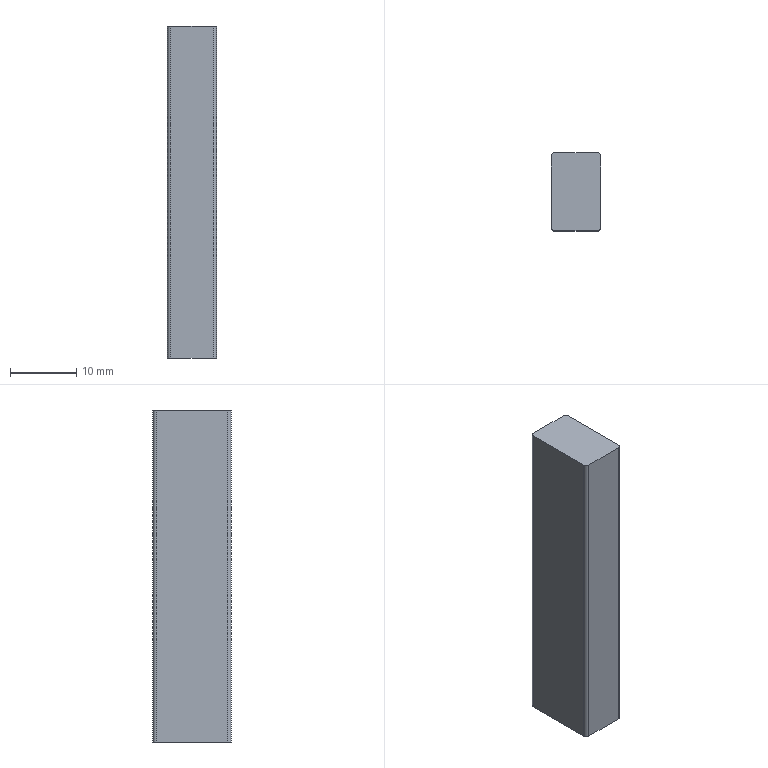Part | NX | features BREP 1 | 1 solid | 10 faces | box 7.385 x 11.783 x 50 mm | volume 4340 mm3 | plane 6 | cylinder 4 | commonest cylinder face diameters 1 x4
STEP:
#1=CARTESIAN_POINT('',(-3.192,5.891,-40.6));
#2=VERTEX_POINT('',#1);
#3=CARTESIAN_POINT('',(-3.692,5.391,-40.6));
#4=VERTEX_POINT('',#3);
#5=CARTESIAN_POINT('',(-3.192,5.391,-40.6));
#6=DIRECTION('',(0.,0.,1.));
#7=DIRECTION('',(1.,0.,0.));
#8=AXIS2_PLACEMENT_3D('',#5,#6,#7);
#9=CIRCLE('',#8,0.5);
#10=EDGE_CURVE('',#2,#4,#9,.T.);
#11=ORIENTED_EDGE('',*,*,#10,.F.);
#12=CARTESIAN_POINT('',(-3.192,5.891,-90.6));
#13=VERTEX_POINT('',#12);
#14=CARTESIAN_POINT('',(-3.192,5.891,-90.6));
#15=DIRECTION('',(0.,0.,1.));
#16=VECTOR('',#15,1000.);
#17=LINE('',#14,#16);
#18=EDGE_CURVE('',#13,#2,#17,.T.);
#19=ORIENTED_EDGE('',*,*,#18,.F.);
#20=CARTESIAN_POINT('',(-3.692,5.391,-90.6));
#21=VERTEX_POINT('',#20);
#22=CARTESIAN_POINT('',(-3.192,5.391,-90.6));
#23=DIRECTION('',(0.,0.,1.));
#24=DIRECTION('',(1.,0.,0.));
#25=AXIS2_PLACEMENT_3D('',#22,#23,#24);
#26=CIRCLE('',#25,0.5);
#27=EDGE_CURVE('',#13,#21,#26,.T.);
#28=ORIENTED_EDGE('',*,*,#27,.T.);
#29=CARTESIAN_POINT('',(-3.692,5.391,-90.6));
#30=DIRECTION('',(0.,0.,1.));
#31=VECTOR('',#30,1000.);
#32=LINE('',#29,#31);
#33=EDGE_CURVE('',#21,#4,#32,.T.);
#34=ORIENTED_EDGE('',*,*,#33,.T.);
#35=EDGE_LOOP('',(#11,#19,#28,#34));
#36=FACE_BOUND('',#35,.T.);
#37=CARTESIAN_POINT('',(-3.192,5.391,-90.6));
#38=DIRECTION('',(0.,0.,1.));
#39=DIRECTION('',(-1.,0.,0.));
#40=AXIS2_PLACEMENT_3D('',#37,#38,#39);
#41=CYLINDRICAL_SURFACE('',#40,0.5);
#42=ADVANCED_FACE('',(#36),#41,.T.);
#43=CARTESIAN_POINT('',(-3.692,-5.391,-40.6));
#44=VERTEX_POINT('',#43);
#45=CARTESIAN_POINT('',(-3.692,-5.391,-40.6));
#46=DIRECTION('',(0.,1.,0.));
#47=VECTOR('',#46,1000.);
#48=LINE('',#45,#47);
#49=EDGE_CURVE('',#44,#4,#48,.T.);
#50=ORIENTED_EDGE('',*,*,#49,.T.);
#51=ORIENTED_EDGE('',*,*,#33,.F.);
#52=CARTESIAN_POINT('',(-3.692,-5.391,-90.6));
#53=VERTEX_POINT('',#52);
#54=CARTESIAN_POINT('',(-3.692,-5.391,-90.6));
#55=DIRECTION('',(0.,1.,0.));
#56=VECTOR('',#55,1000.);
#57=LINE('',#54,#56);
#58=EDGE_CURVE('',#53,#21,#57,.T.);
#59=ORIENTED_EDGE('',*,*,#58,.F.);
#60=CARTESIAN_POINT('',(-3.692,-5.391,-90.6));
#61=DIRECTION('',(0.,0.,1.));
#62=VECTOR('',#61,1000.);
#63=LINE('',#60,#62);
#64=EDGE_CURVE('',#53,#44,#63,.T.);
#65=ORIENTED_EDGE('',*,*,#64,.T.);
#66=EDGE_LOOP('',(#50,#51,#59,#65));
#67=FACE_BOUND('',#66,.T.);
#68=CARTESIAN_POINT('',(-3.692,-5.391,-90.6));
#69=DIRECTION('',(1.,0.,0.));
#70=DIRECTION('',(0.,-1.,0.));
#71=AXIS2_PLACEMENT_3D('',#68,#69,#70);
#72=PLANE('',#71);
#73=ADVANCED_FACE('',(#67),#72,.F.);
#74=CARTESIAN_POINT('',(-3.192,-5.891,-40.6));
#75=VERTEX_POINT('',#74);
#76=CARTESIAN_POINT('',(-3.192,-5.391,-40.6));
#77=DIRECTION('',(0.,0.,1.));
#78=DIRECTION('',(1.,0.,0.));
#79=AXIS2_PLACEMENT_3D('',#76,#77,#78);
#80=CIRCLE('',#79,0.5);
#81=EDGE_CURVE('',#44,#75,#80,.T.);
#82=ORIENTED_EDGE('',*,*,#81,.F.);
#83=ORIENTED_EDGE('',*,*,#64,.F.);
#84=CARTESIAN_POINT('',(-3.192,-5.891,-90.6));
#85=VERTEX_POINT('',#84);
#86=CARTESIAN_POINT('',(-3.192,-5.391,-90.6));
#87=DIRECTION('',(0.,0.,1.));
#88=DIRECTION('',(1.,0.,0.));
#89=AXIS2_PLACEMENT_3D('',#86,#87,#88);
#90=CIRCLE('',#89,0.5);
#91=EDGE_CURVE('',#53,#85,#90,.T.);
#92=ORIENTED_EDGE('',*,*,#91,.T.);
#93=CARTESIAN_POINT('',(-3.192,-5.891,-90.6));
#94=DIRECTION('',(0.,0.,1.));
#95=VECTOR('',#94,1000.);
#96=LINE('',#93,#95);
#97=EDGE_CURVE('',#85,#75,#96,.T.);
#98=ORIENTED_EDGE('',*,*,#97,.T.);
#99=EDGE_LOOP('',(#82,#83,#92,#98));
#100=FACE_BOUND('',#99,.T.);
#101=CARTESIAN_POINT('',(-3.192,-5.391,-90.6));
#102=DIRECTION('',(0.,0.,1.));
#103=DIRECTION('',(-1.,0.,0.));
#104=AXIS2_PLACEMENT_3D('',#101,#102,#103);
#105=CYLINDRICAL_SURFACE('',#104,0.5);
#106=ADVANCED_FACE('',(#100),#105,.T.);
#107=CARTESIAN_POINT('',(3.192,-5.891,-40.6));
#108=VERTEX_POINT('',#107);
#109=CARTESIAN_POINT('',(3.192,-5.891,-40.6));
#110=DIRECTION('',(-1.,0.,0.));
#111=VECTOR('',#110,1000.);
#112=LINE('',#109,#111);
#113=EDGE_CURVE('',#108,#75,#112,.T.);
#114=ORIENTED_EDGE('',*,*,#113,.T.);
#115=ORIENTED_EDGE('',*,*,#97,.F.);
#116=CARTESIAN_POINT('',(3.192,-5.891,-90.6));
#117=VERTEX_POINT('',#116);
#118=CARTESIAN_POINT('',(3.192,-5.891,-90.6));
#119=DIRECTION('',(-1.,0.,0.));
#120=VECTOR('',#119,1000.);
#121=LINE('',#118,#120);
#122=EDGE_CURVE('',#117,#85,#121,.T.);
#123=ORIENTED_EDGE('',*,*,#122,.F.);
#124=CARTESIAN_POINT('',(3.192,-5.891,-90.6));
#125=DIRECTION('',(0.,0.,1.));
#126=VECTOR('',#125,1000.);
#127=LINE('',#124,#126);
#128=EDGE_CURVE('',#117,#108,#127,.T.);
#129=ORIENTED_EDGE('',*,*,#128,.T.);
#130=EDGE_LOOP('',(#114,#115,#123,#129));
#131=FACE_BOUND('',#130,.T.);
#132=CARTESIAN_POINT('',(3.192,-5.891,-90.6));
#133=DIRECTION('',(0.,1.,0.));
#134=DIRECTION('',(0.,0.,-1.));
#135=AXIS2_PLACEMENT_3D('',#132,#133,#134);
#136=PLANE('',#135);
#137=ADVANCED_FACE('',(#131),#136,.F.);
#138=CARTESIAN_POINT('',(3.692,-5.391,-40.6));
#139=VERTEX_POINT('',#138);
#140=CARTESIAN_POINT('',(3.192,-5.391,-40.6));
#141=DIRECTION('',(0.,0.,1.));
#142=DIRECTION('',(1.,0.,0.));
#143=AXIS2_PLACEMENT_3D('',#140,#141,#142);
#144=CIRCLE('',#143,0.5);
#145=EDGE_CURVE('',#108,#139,#144,.T.);
#146=ORIENTED_EDGE('',*,*,#145,.F.);
#147=ORIENTED_EDGE('',*,*,#128,.F.);
#148=CARTESIAN_POINT('',(3.692,-5.391,-90.6));
#149=VERTEX_POINT('',#148);
#150=CARTESIAN_POINT('',(3.192,-5.391,-90.6));
#151=DIRECTION('',(0.,0.,1.));
#152=DIRECTION('',(1.,0.,0.));
#153=AXIS2_PLACEMENT_3D('',#150,#151,#152);
#154=CIRCLE('',#153,0.5);
#155=EDGE_CURVE('',#117,#149,#154,.T.);
#156=ORIENTED_EDGE('',*,*,#155,.T.);
#157=CARTESIAN_POINT('',(3.692,-5.391,-90.6));
#158=DIRECTION('',(0.,0.,1.));
#159=VECTOR('',#158,1000.);
#160=LINE('',#157,#159);
#161=EDGE_CURVE('',#149,#139,#160,.T.);
#162=ORIENTED_EDGE('',*,*,#161,.T.);
#163=EDGE_LOOP('',(#146,#147,#156,#162));
#164=FACE_BOUND('',#163,.T.);
#165=CARTESIAN_POINT('',(3.192,-5.391,-90.6));
#166=DIRECTION('',(0.,0.,1.));
#167=DIRECTION('',(-1.,0.,0.));
#168=AXIS2_PLACEMENT_3D('',#165,#166,#167);
#169=CYLINDRICAL_SURFACE('',#168,0.5);
#170=ADVANCED_FACE('',(#164),#169,.T.);
#171=CARTESIAN_POINT('',(3.692,5.391,-40.6));
#172=VERTEX_POINT('',#171);
#173=CARTESIAN_POINT('',(3.692,5.391,-40.6));
#174=DIRECTION('',(0.,-1.,0.));
#175=VECTOR('',#174,1000.);
#176=LINE('',#173,#175);
#177=EDGE_CURVE('',#172,#139,#176,.T.);
#178=ORIENTED_EDGE('',*,*,#177,.T.);
#179=ORIENTED_EDGE('',*,*,#161,.F.);
#180=CARTESIAN_POINT('',(3.692,5.391,-90.6));
#181=VERTEX_POINT('',#180);
#182=CARTESIAN_POINT('',(3.692,5.391,-90.6));
#183=DIRECTION('',(0.,-1.,0.));
#184=VECTOR('',#183,1000.);
#185=LINE('',#182,#184);
#186=EDGE_CURVE('',#181,#149,#185,.T.);
#187=ORIENTED_EDGE('',*,*,#186,.F.);
#188=CARTESIAN_POINT('',(3.692,5.391,-90.6));
#189=DIRECTION('',(0.,0.,1.));
#190=VECTOR('',#189,1000.);
#191=LINE('',#188,#190);
#192=EDGE_CURVE('',#181,#172,#191,.T.);
#193=ORIENTED_EDGE('',*,*,#192,.T.);
#194=EDGE_LOOP('',(#178,#179,#187,#193));
#195=FACE_BOUND('',#194,.T.);
#196=CARTESIAN_POINT('',(3.692,5.391,-90.6));
#197=DIRECTION('',(-1.,0.,0.));
#198=DIRECTION('',(0.,0.,-1.));
#199=AXIS2_PLACEMENT_3D('',#196,#197,#198);
#200=PLANE('',#199);
#201=ADVANCED_FACE('',(#195),#200,.F.);
#202=CARTESIAN_POINT('',(3.192,5.891,-40.6));
#203=VERTEX_POINT('',#202);
#204=CARTESIAN_POINT('',(3.192,5.391,-40.6));
#205=DIRECTION('',(0.,0.,1.));
#206=DIRECTION('',(1.,0.,0.));
#207=AXIS2_PLACEMENT_3D('',#204,#205,#206);
#208=CIRCLE('',#207,0.5);
#209=EDGE_CURVE('',#172,#203,#208,.T.);
#210=ORIENTED_EDGE('',*,*,#209,.F.);
#211=ORIENTED_EDGE('',*,*,#192,.F.);
#212=CARTESIAN_POINT('',(3.192,5.891,-90.6));
#213=VERTEX_POINT('',#212);
#214=CARTESIAN_POINT('',(3.192,5.391,-90.6));
#215=DIRECTION('',(0.,0.,1.));
#216=DIRECTION('',(1.,0.,0.));
#217=AXIS2_PLACEMENT_3D('',#214,#215,#216);
#218=CIRCLE('',#217,0.5);
#219=EDGE_CURVE('',#181,#213,#218,.T.);
#220=ORIENTED_EDGE('',*,*,#219,.T.);
#221=CARTESIAN_POINT('',(3.192,5.891,-90.6));
#222=DIRECTION('',(0.,0.,1.));
#223=VECTOR('',#222,1000.);
#224=LINE('',#221,#223);
#225=EDGE_CURVE('',#213,#203,#224,.T.);
#226=ORIENTED_EDGE('',*,*,#225,.T.);
#227=EDGE_LOOP('',(#210,#211,#220,#226));
#228=FACE_BOUND('',#227,.T.);
#229=CARTESIAN_POINT('',(3.192,5.391,-90.6));
#230=DIRECTION('',(0.,0.,1.));
#231=DIRECTION('',(-1.,0.,0.));
#232=AXIS2_PLACEMENT_3D('',#229,#230,#231);
#233=CYLINDRICAL_SURFACE('',#232,0.5);
#234=ADVANCED_FACE('',(#228),#233,.T.);
#235=CARTESIAN_POINT('',(-3.192,5.891,-40.6));
#236=DIRECTION('',(1.,0.,0.));
#237=VECTOR('',#236,1000.);
#238=LINE('',#235,#237);
#239=EDGE_CURVE('',#2,#203,#238,.T.);
#240=ORIENTED_EDGE('',*,*,#239,.T.);
#241=ORIENTED_EDGE('',*,*,#225,.F.);
#242=CARTESIAN_POINT('',(-3.192,5.891,-90.6));
#243=DIRECTION('',(1.,0.,0.));
#244=VECTOR('',#243,1000.);
#245=LINE('',#242,#244);
#246=EDGE_CURVE('',#13,#213,#245,.T.);
#247=ORIENTED_EDGE('',*,*,#246,.F.);
#248=ORIENTED_EDGE('',*,*,#18,.T.);
#249=EDGE_LOOP('',(#240,#241,#247,#248));
#250=FACE_BOUND('',#249,.T.);
#251=CARTESIAN_POINT('',(-3.192,5.891,-90.6));
#252=DIRECTION('',(0.,-1.,0.));
#253=DIRECTION('',(0.,0.,1.));
#254=AXIS2_PLACEMENT_3D('',#251,#252,#253);
#255=PLANE('',#254);
#256=ADVANCED_FACE('',(#250),#255,.F.);
#257=ORIENTED_EDGE('',*,*,#27,.F.);
#258=ORIENTED_EDGE('',*,*,#246,.T.);
#259=ORIENTED_EDGE('',*,*,#219,.F.);
#260=ORIENTED_EDGE('',*,*,#186,.T.);
#261=ORIENTED_EDGE('',*,*,#155,.F.);
#262=ORIENTED_EDGE('',*,*,#122,.T.);
#263=ORIENTED_EDGE('',*,*,#91,.F.);
#264=ORIENTED_EDGE('',*,*,#58,.T.);
#265=EDGE_LOOP('',(#257,#258,#259,#260,#261,#262,#263,#264));
#266=FACE_BOUND('',#265,.T.);
#267=CARTESIAN_POINT('',(-3.192,5.391,-90.6));
#268=DIRECTION('',(0.,0.,1.));
#269=DIRECTION('',(-1.,0.,0.));
#270=AXIS2_PLACEMENT_3D('',#267,#268,#269);
#271=PLANE('',#270);
#272=ADVANCED_FACE('',(#266),#271,.F.);
#273=ORIENTED_EDGE('',*,*,#10,.T.);
#274=ORIENTED_EDGE('',*,*,#49,.F.);
#275=ORIENTED_EDGE('',*,*,#81,.T.);
#276=ORIENTED_EDGE('',*,*,#113,.F.);
#277=ORIENTED_EDGE('',*,*,#145,.T.);
#278=ORIENTED_EDGE('',*,*,#177,.F.);
#279=ORIENTED_EDGE('',*,*,#209,.T.);
#280=ORIENTED_EDGE('',*,*,#239,.F.);
#281=EDGE_LOOP('',(#273,#274,#275,#276,#277,#278,#279,#280));
#282=FACE_BOUND('',#281,.T.);
#283=CARTESIAN_POINT('',(-3.192,5.391,-40.6));
#284=DIRECTION('',(0.,0.,1.));
#285=DIRECTION('',(-1.,0.,0.));
#286=AXIS2_PLACEMENT_3D('',#283,#284,#285);
#287=PLANE('',#286);
#288=ADVANCED_FACE('',(#282),#287,.T.);
#289=CLOSED_SHELL('',(#42,#73,#106,#137,#170,#201,#234,#256,#272,#288));
#290=MANIFOLD_SOLID_BREP('',#289);
#291=(LENGTH_UNIT()NAMED_UNIT(*)SI_UNIT(.MILLI.,.METRE.));
#292=UNCERTAINTY_MEASURE_WITH_UNIT(LENGTH_MEASURE(0.00001),#291,'','');
#293=(NAMED_UNIT(*)PLANE_ANGLE_UNIT()SI_UNIT($,.RADIAN.));
#294=(NAMED_UNIT(*)SI_UNIT($,.STERADIAN.)SOLID_ANGLE_UNIT());
#295=(GEOMETRIC_REPRESENTATION_CONTEXT(3)GLOBAL_UNCERTAINTY_ASSIGNED_CONTEXT((#292))GLOBAL_UNIT_ASSIGNED_CONTEXT((#291,#293,#294))REPRESENTATION_CONTEXT('',''));
#296=ADVANCED_BREP_SHAPE_REPRESENTATION('',(#290),#295);